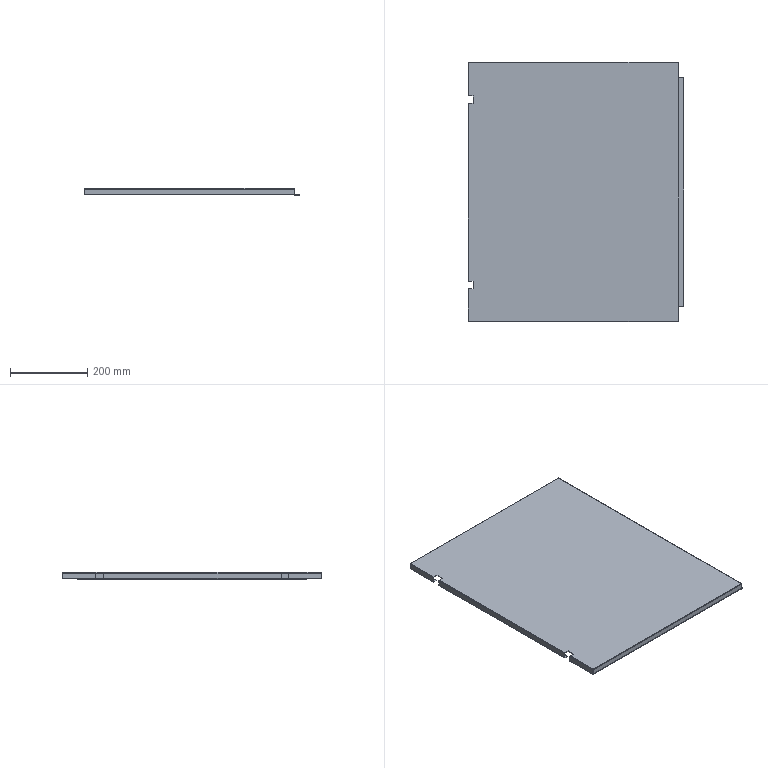Part | SolidWorks | 1 solid | 124 faces | box 559 x 672 x 18.5 mm | volume 634923 mm3 | plane 88 | cylinder 28 | spline 8 | commonest cylinder face diameters 0.2 x12 3.2 x12 6 x4